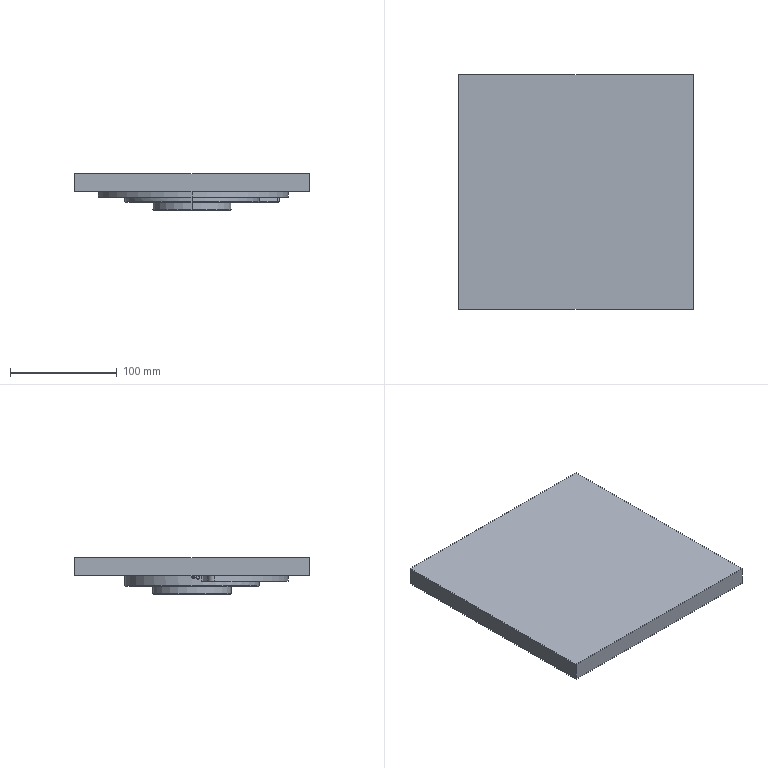NC program | NX | posted with a generic post | part box 220 x 220 x 34.5 mm
Lines 3232 to 4489 of 14163:
(ZLEVEL_PROFILE_COPY , TOOL : D10JING)
N6426 T07 M6
N6428 G54
N6430 G17 G0 G90 X93.952 Y24.124 S8000 M3
N6432 G43 Z30. H7
N6434 Z-17.
N6436 G94 G1 X92.706 Y22.948 F1200.
N6438 G3 X92.42 Y21.99 R1.
N6440 G1 X92.427 Y21.958
N6442 G2 X84.432 Y9.81 R10.
N6444 G1 X67.654 Y6.852
N6446 X67.704 Y6.339
N6448 G2 X-54.559 Y-40.587 R68.
N6450 G1 X-54.815 Y-40.238
N6452 X-54.822 Y-40.231
N6454 G2 X-56.208 Y-38.271 R68.
N6456 G1 X-56.229 Y-38.238
N6458 X-70.985 Y-46.757
N6460 G2 X-84.924 Y-42.578 R10.
N6462 G3 X-85.759 Y-42.028 R1.
N6464 G1 X-87.471 Y-41.927
N6466 G0 Z30.
N6468 M5
(ZLEVEL_PROFILE_COPY_1 , TOOL : D6)
N6470 T09 M6
N6472 G54
N6474 G17 G0 G90 X44.19 Y25.815 S9500 M3
N6476 G43 Z30. H9
N6478 Z-0.493
N6480 G94 G1 X43.248 Y26.254 F1000.
N6482 G3 X42.65 Y26.202 R0.6
N6484 G1 X40.963 Y25.02 F1500.
N6486 G2 X41.984 Y23.268 R48.
N6488 G3 X42.498 Y22.959 R0.6
N6490 G1 X43.512 Y22.941
N6492 G0 X44.19 Y25.815 Z-0.986
N6494 G1 X43.248 Y26.254 F1000.
N6496 G3 X42.65 Y26.202 R0.6
N6498 G1 X40.963 Y25.02 F1500.
N6500 G2 X41.984 Y23.268 R48.
N6502 G3 X42.498 Y22.959 R0.6
N6504 G1 X43.512 Y22.941
N6506 G0 X44.19 Y25.815 Z-1.479
N6508 G1 X43.248 Y26.254 F1000.
N6510 G3 X42.65 Y26.202 R0.6
N6512 G1 X40.963 Y25.02 F1500.
N6514 G2 X41.984 Y23.268 R48.
N6516 G3 X42.498 Y22.959 R0.6
N6518 G1 X43.512 Y22.941
N6520 G0 X44.19 Y25.815 Z-1.972
N6522 G1 X43.248 Y26.254 F1000.
N6524 G3 X42.65 Y26.202 R0.6
N6526 G1 X40.963 Y25.02 F1500.
N6528 G2 X41.984 Y23.268 R48.
N6530 G3 X42.498 Y22.959 R0.6
N6532 G1 X43.512 Y22.941
N6534 G0 X44.19 Y25.815 Z-2.465
N6536 G1 X43.248 Y26.254 F1000.
N6538 G3 X42.65 Y26.202 R0.6
N6540 G1 X40.963 Y25.02 F1500.
N6542 G2 X41.984 Y23.268 R48.
N6544 G3 X42.498 Y22.959 R0.6
N6546 G1 X43.512 Y22.941
N6548 G0 X44.19 Y25.815 Z-2.958
N6550 G1 X43.248 Y26.254 F1000.
N6552 G3 X42.65 Y26.202 R0.6
N6554 G1 X40.963 Y25.02 F1500.
N6556 G2 X41.984 Y23.268 R48.
N6558 G3 X42.498 Y22.959 R0.6
N6560 G1 X43.512 Y22.941
N6562 G0 X44.19 Y25.815 Z-3.451
N6564 G1 X43.248 Y26.254 F1000.
N6566 G3 X42.65 Y26.202 R0.6
N6568 G1 X40.963 Y25.02 F1500.
N6570 G2 X41.984 Y23.268 R48.
N6572 G3 X42.498 Y22.959 R0.6
N6574 G1 X43.512 Y22.941
N6576 G0 X44.19 Y25.815 Z-3.944
N6578 G1 X43.248 Y26.254 F1000.
N6580 G3 X42.65 Y26.202 R0.6
N6582 G1 X40.963 Y25.02 F1500.
N6584 G2 X41.984 Y23.268 R48.
N6586 G3 X42.498 Y22.959 R0.6
N6588 G1 X43.512 Y22.941
N6590 G0 X44.19 Y25.815 Z-4.438
N6592 G1 X43.248 Y26.254 F1000.
N6594 G3 X42.65 Y26.202 R0.6
N6596 G1 X40.963 Y25.02 F1500.
N6598 G2 X41.984 Y23.268 R48.
N6600 G3 X42.498 Y22.959 R0.6
N6602 G1 X43.512 Y22.941
N6604 G0 X44.19 Y25.815 Z-4.931
N6606 G1 X43.248 Y26.254 F1000.
N6608 G3 X42.65 Y26.202 R0.6
N6610 G1 X40.963 Y25.02 F1500.
N6612 G2 X41.984 Y23.268 R48.
N6614 G3 X42.498 Y22.959 R0.6
N6616 G1 X43.512 Y22.941
N6618 G0 X44.19 Y25.815 Z-5.424
N6620 G1 X43.248 Y26.254 F1000.
N6622 G3 X42.65 Y26.202 R0.6
N6624 G1 X40.963 Y25.02 F1500.
N6626 G2 X41.984 Y23.268 R48.
N6628 G3 X42.498 Y22.959 R0.6
N6630 G1 X43.512 Y22.941
N6632 G0 X44.19 Y25.815 Z-5.917
N6634 G1 X43.248 Y26.254 F1000.
N6636 G3 X42.65 Y26.202 R0.6
N6638 G1 X40.963 Y25.02 F1500.
N6640 G2 X41.984 Y23.268 R48.
N6642 G3 X42.498 Y22.959 R0.6
N6644 G1 X43.512 Y22.941
N6646 G0 X44.19 Y25.815 Z-6.41
N6648 G1 X43.248 Y26.254 F1000.
N6650 G3 X42.65 Y26.202 R0.6
N6652 G1 X40.963 Y25.02 F1500.
N6654 G2 X41.984 Y23.268 R48.
N6656 G3 X42.498 Y22.959 R0.6
N6658 G1 X43.512 Y22.941
N6660 G0 X44.19 Y25.815 Z-6.903
N6662 G1 X43.248 Y26.254 F1000.
N6664 G3 X42.65 Y26.202 R0.6
N6666 G1 X40.963 Y25.02 F1500.
N6668 G2 X41.984 Y23.268 R48.
N6670 G3 X42.498 Y22.959 R0.6
N6672 G1 X43.512 Y22.941
N6674 G0 X44.19 Y25.815 Z-7.396
N6676 G1 X43.248 Y26.254 F1000.
N6678 G3 X42.65 Y26.202 R0.6
N6680 G1 X40.963 Y25.02 F1500.
N6682 G2 X41.984 Y23.268 R48.
N6684 G3 X42.498 Y22.959 R0.6
N6686 G1 X43.512 Y22.941
N6688 G0 X44.19 Y25.815 Z-7.889
N6690 G1 X43.248 Y26.254 F1000.
N6692 G3 X42.65 Y26.202 R0.6
N6694 G1 X40.963 Y25.02 F1500.
N6696 G2 X41.984 Y23.268 R48.
N6698 G3 X42.498 Y22.959 R0.6
N6700 G1 X43.512 Y22.941
N6702 G0 X44.19 Y25.815 Z-8.382
N6704 G1 X43.248 Y26.254 F1000.
N6706 G3 X42.65 Y26.202 R0.6
N6708 G1 X40.963 Y25.02 F1500.
N6710 G2 X41.984 Y23.268 R48.
N6712 G3 X42.498 Y22.959 R0.6
N6714 G1 X43.512 Y22.941
N6716 G0 X44.19 Y25.815 Z-8.875
N6718 G1 X43.248 Y26.254 F1000.
N6720 G3 X42.65 Y26.202 R0.6
N6722 G1 X40.963 Y25.02 F1500.
N6724 G2 X41.984 Y23.268 R48.
N6726 G3 X42.498 Y22.959 R0.6
N6728 G1 X43.512 Y22.941
N6730 G0 X44.19 Y25.815 Z-9.25
N6732 G1 X43.248 Y26.254 F1000.
N6734 G3 X42.65 Y26.202 R0.6
N6736 G1 X40.963 Y25.02 F1500.
N6738 G2 X41.984 Y23.268 R48.
N6740 G3 X42.498 Y22.959 R0.6
N6742 G1 X43.512 Y22.941
N6744 G0 X44.19 Y25.815 Z-9.625
N6746 G1 X43.248 Y26.254 F1000.
N6748 G3 X42.65 Y26.202 R0.6
N6750 G1 X40.963 Y25.02 F1500.
N6752 G2 X41.984 Y23.268 R48.
N6754 G3 X42.498 Y22.959 R0.6
N6756 G1 X43.512 Y22.941
N6758 G0 X44.19 Y25.815 Z-10.
N6760 G1 X43.248 Y26.254 F1000.
N6762 G3 X42.65 Y26.202 R0.6
N6764 G1 X40.963 Y25.02 F1500.
N6766 G2 X41.984 Y23.268 R48.
N6768 G3 X42.498 Y22.959 R0.6
N6770 G1 X43.512 Y22.941
N6772 G0 Z30.
N6774 X39.192 Y14.12
N6776 Z-0.493
N6778 G1 X38.335 Y14.707 F1000.
N6780 G3 X37.737 Y14.753 R0.6
N6782 G1 X35.912 Y13.878 F1500.
N6784 G2 X36.579 Y12.008 R38.5
N6786 G3 X37.027 Y11.608 R0.6
N6788 G1 X38.029 Y11.398
N6790 G0 X39.192 Y14.12 Z-0.986
N6792 G1 X38.335 Y14.707 F1000.
N6794 G3 X37.737 Y14.753 R0.6
N6796 G1 X35.912 Y13.878 F1500.
N6798 G2 X36.579 Y12.008 R38.5
N6800 G3 X37.026 Y11.608 R0.6
N6802 G1 X38.028 Y11.399
N6804 G0 X39.192 Y14.12 Z-1.479
N6806 G1 X38.335 Y14.707 F1000.
N6808 G3 X37.737 Y14.753 R0.6
N6810 G1 X35.912 Y13.878 F1500.
N6812 G2 X36.579 Y12.008 R38.5
N6814 G3 X37.026 Y11.608 R0.6
N6816 G1 X38.028 Y11.398
N6818 G0 X39.192 Y14.12 Z-1.972
N6820 G1 X38.335 Y14.707 F1000.
N6822 G3 X37.737 Y14.753 R0.6
N6824 G1 X35.912 Y13.878 F1500.
N6826 G2 X36.579 Y12.008 R38.5
N6828 G3 X37.026 Y11.608 R0.6
N6830 G1 X38.028 Y11.398
N6832 G0 X39.193 Y14.12 Z-2.465
N6834 G1 X38.335 Y14.707 F1000.
N6836 G3 X37.737 Y14.753 R0.6
N6838 G1 X35.912 Y13.878 F1500.
N6840 G2 X36.579 Y12.008 R38.5
N6842 G3 X37.026 Y11.608 R0.6
N6844 G1 X38.029 Y11.398
N6846 G0 X39.193 Y14.12 Z-2.958
N6848 G1 X38.335 Y14.707 F1000.
N6850 G3 X37.737 Y14.753 R0.6
N6852 G1 X35.912 Y13.878 F1500.
N6854 G2 X36.579 Y12.008 R38.5
N6856 G3 X37.026 Y11.608 R0.6
N6858 G1 X38.029 Y11.398
N6860 G0 X39.193 Y14.12 Z-3.451
N6862 G1 X38.335 Y14.707 F1000.
N6864 G3 X37.737 Y14.753 R0.6
N6866 G1 X35.912 Y13.878 F1500.
N6868 G2 X36.579 Y12.008 R38.5
N6870 G3 X37.027 Y11.608 R0.6
N6872 G1 X38.029 Y11.398
N6874 G0 X39.193 Y14.12 Z-3.944
N6876 G1 X38.335 Y14.707 F1000.
N6878 G3 X37.737 Y14.753 R0.6
N6880 G1 X35.912 Y13.878 F1500.
N6882 G2 X36.579 Y12.008 R38.5
N6884 G3 X37.027 Y11.608 R0.6
N6886 G1 X38.029 Y11.398
N6888 G0 X39.193 Y14.12 Z-4.438
N6890 G1 X38.335 Y14.707 F1000.
N6892 G3 X37.737 Y14.753 R0.6
N6894 G1 X35.912 Y13.878 F1500.
N6896 G2 X36.579 Y12.008 R38.5
N6898 G3 X37.027 Y11.608 R0.6
N6900 G1 X38.029 Y11.398
N6902 G0 X39.193 Y14.12 Z-4.931
N6904 G1 X38.335 Y14.707 F1000.
N6906 G3 X37.737 Y14.753 R0.6
N6908 G1 X35.912 Y13.878 F1500.
N6910 G2 X36.579 Y12.008 R38.5
N6912 G3 X37.027 Y11.608 R0.6
N6914 G1 X38.029 Y11.398
N6916 G0 X39.193 Y14.12 Z-5.424
N6918 G1 X38.335 Y14.707 F1000.
N6920 G3 X37.737 Y14.753 R0.6
N6922 G1 X35.912 Y13.878 F1500.
N6924 G2 X36.579 Y12.008 R38.5
N6926 G3 X37.027 Y11.608 R0.6
N6928 G1 X38.029 Y11.398
N6930 G0 X39.193 Y14.12 Z-5.917
N6932 G1 X38.335 Y14.707 F1000.
N6934 G3 X37.737 Y14.753 R0.6
N6936 G1 X35.912 Y13.878 F1500.
N6938 G2 X36.579 Y12.008 R38.5
N6940 G3 X37.027 Y11.608 R0.6
N6942 G1 X38.029 Y11.398
N6944 G0 X39.193 Y14.12 Z-6.41
N6946 G1 X38.335 Y14.707 F1000.
N6948 G3 X37.737 Y14.753 R0.6
N6950 G1 X35.912 Y13.878 F1500.
N6952 G2 X36.58 Y12.008 R38.5
N6954 G3 X37.027 Y11.608 R0.6
N6956 G1 X38.029 Y11.398
N6958 G0 X39.193 Y14.12 Z-6.903
N6960 G1 X38.336 Y14.707 F1000.
N6962 G3 X37.737 Y14.753 R0.6
N6964 G1 X35.912 Y13.878 F1500.
N6966 G2 X36.58 Y12.008 R38.5
N6968 G3 X37.027 Y11.608 R0.6
N6970 G1 X38.029 Y11.398
N6972 G0 X39.193 Y14.12 Z-7.396
N6974 G1 X38.336 Y14.707 F1000.
N6976 G3 X37.737 Y14.753 R0.6
N6978 G1 X35.912 Y13.878 F1500.
N6980 G2 X36.58 Y12.008 R38.5
N6982 G3 X37.027 Y11.608 R0.6
N6984 G1 X38.029 Y11.398
N6986 G0 X39.193 Y14.12 Z-7.889
N6988 G1 X38.336 Y14.707 F1000.
N6990 G3 X37.737 Y14.753 R0.6
N6992 G1 X35.912 Y13.878 F1500.
N6994 G2 X36.58 Y12.008 R38.5
N6996 G3 X37.027 Y11.608 R0.6
N6998 G1 X38.029 Y11.398
N7000 G0 X39.193 Y14.12 Z-8.382
N7002 G1 X38.336 Y14.707 F1000.
N7004 G3 X37.737 Y14.753 R0.6
N7006 G1 X35.912 Y13.878 F1500.
N7008 G2 X36.58 Y12.008 R38.5
N7010 G3 X37.027 Y11.608 R0.6
N7012 G1 X38.029 Y11.398
N7014 G0 X39.193 Y14.12 Z-8.875
N7016 G1 X38.336 Y14.707 F1000.
N7018 G3 X37.737 Y14.753 R0.6
N7020 G1 X35.912 Y13.878 F1500.
N7022 G2 X36.58 Y12.008 R38.5
N7024 G3 X37.027 Y11.608 R0.6
N7026 G1 X38.029 Y11.398
N7028 G0 X39.193 Y14.12 Z-9.25
N7030 G1 X38.336 Y14.707 F1000.
N7032 G3 X37.738 Y14.753 R0.6
N7034 G1 X35.912 Y13.878 F1500.
N7036 G2 X36.58 Y12.008 R38.5
N7038 G3 X37.027 Y11.608 R0.6
N7040 G1 X38.029 Y11.398
N7042 G0 X39.193 Y14.12 Z-9.625
N7044 G1 X38.336 Y14.707 F1000.
N7046 G3 X37.738 Y14.753 R0.6
N7048 G1 X35.912 Y13.878 F1500.
N7050 G2 X36.58 Y12.008 R38.5
N7052 G3 X37.027 Y11.607 R0.6
N7054 G1 X38.029 Y11.398
N7056 G0 X39.193 Y14.12 Z-10.
N7058 G1 X38.336 Y14.707 F1000.
N7060 G3 X37.738 Y14.753 R0.6
N7062 G1 X35.912 Y13.878 F1500.
N7064 G2 X36.58 Y12.008 R38.5
N7066 G3 X37.027 Y11.607 R0.6
N7068 G1 X38.029 Y11.398
N7070 G0 Z30.
N7072 X-11.399 Y-38.028
N7074 Z-0.493
N7076 G1 X-11.608 Y-37.026 F1000.
N7078 G3 X-12.009 Y-36.579 R0.6
N7080 G2 X-13.878 Y-35.912 R38.5 F1500.
N7082 G1 X-14.753 Y-37.737
N7084 G3 X-14.707 Y-38.335 R0.6
N7086 G1 X-14.12 Y-39.192
N7088 G0 X-11.399 Y-38.028 Z-0.986
N7090 G1 X-11.608 Y-37.026 F1000.
N7092 G3 X-12.009 Y-36.579 R0.6
N7094 G2 X-13.878 Y-35.912 R38.5 F1500.
N7096 G1 X-14.753 Y-37.737
N7098 G3 X-14.707 Y-38.335 R0.6
N7100 G1 X-14.12 Y-39.192
N7102 G0 X-11.399 Y-38.028 Z-1.479
N7104 G1 X-11.608 Y-37.026 F1000.
N7106 G3 X-12.009 Y-36.579 R0.6
N7108 G2 X-13.878 Y-35.912 R38.5 F1500.
N7110 G1 X-14.753 Y-37.737
N7112 G3 X-14.707 Y-38.335 R0.6
N7114 G1 X-14.12 Y-39.192
N7116 G0 X-11.399 Y-38.028 Z-1.972
N7118 G1 X-11.608 Y-37.026 F1000.
N7120 G3 X-12.009 Y-36.579 R0.6
N7122 G2 X-13.878 Y-35.912 R38.5 F1500.
N7124 G1 X-14.753 Y-37.737
N7126 G3 X-14.707 Y-38.335 R0.6
N7128 G1 X-14.12 Y-39.192
N7130 G0 X-11.399 Y-38.028 Z-2.465
N7132 G1 X-11.608 Y-37.026 F1000.
N7134 G3 X-12.009 Y-36.579 R0.6
N7136 G2 X-13.878 Y-35.912 R38.5 F1500.
N7138 G1 X-14.753 Y-37.737
N7140 G3 X-14.707 Y-38.335 R0.6
N7142 G1 X-14.12 Y-39.192
N7144 G0 X-11.399 Y-38.028 Z-2.958
N7146 G1 X-11.608 Y-37.026 F1000.
N7148 G3 X-12.009 Y-36.579 R0.6
N7150 G2 X-13.878 Y-35.912 R38.5 F1500.
N7152 G1 X-14.753 Y-37.737
N7154 G3 X-14.707 Y-38.335 R0.6
N7156 G1 X-14.12 Y-39.192
N7158 G0 X-11.399 Y-38.028 Z-3.451
N7160 G1 X-11.608 Y-37.026 F1000.
N7162 G3 X-12.009 Y-36.579 R0.6
N7164 G2 X-13.878 Y-35.912 R38.5 F1500.
N7166 G1 X-14.753 Y-37.737
N7168 G3 X-14.707 Y-38.335 R0.6
N7170 G1 X-14.12 Y-39.192
N7172 G0 X-11.399 Y-38.028 Z-3.944
N7174 G1 X-11.608 Y-37.026 F1000.
N7176 G3 X-12.009 Y-36.579 R0.6
N7178 G2 X-13.878 Y-35.912 R38.5 F1500.
N7180 G1 X-14.753 Y-37.737
N7182 G3 X-14.707 Y-38.335 R0.6
N7184 G1 X-14.12 Y-39.192
N7186 G0 X-11.399 Y-38.028 Z-4.438
N7188 G1 X-11.608 Y-37.026 F1000.
N7190 G3 X-12.009 Y-36.579 R0.6
N7192 G2 X-13.878 Y-35.912 R38.5 F1500.
N7194 G1 X-14.753 Y-37.737
N7196 G3 X-14.707 Y-38.335 R0.6
N7198 G1 X-14.12 Y-39.192
N7200 G0 X-11.399 Y-38.028 Z-4.931
N7202 G1 X-11.608 Y-37.026 F1000.
N7204 G3 X-12.009 Y-36.579 R0.6
N7206 G2 X-13.878 Y-35.912 R38.5 F1500.
N7208 G1 X-14.753 Y-37.737
N7210 G3 X-14.707 Y-38.335 R0.6
N7212 G1 X-14.12 Y-39.192
N7214 G0 X-11.399 Y-38.028 Z-5.424
N7216 G1 X-11.608 Y-37.026 F1000.
N7218 G3 X-12.009 Y-36.579 R0.6
N7220 G2 X-13.878 Y-35.912 R38.5 F1500.
N7222 G1 X-14.753 Y-37.737
N7224 G3 X-14.707 Y-38.335 R0.6
N7226 G1 X-14.12 Y-39.192
N7228 G0 X-11.399 Y-38.028 Z-5.917
N7230 G1 X-11.608 Y-37.026 F1000.
N7232 G3 X-12.009 Y-36.579 R0.6
N7234 G2 X-13.878 Y-35.912 R38.5 F1500.
N7236 G1 X-14.753 Y-37.737
N7238 G3 X-14.707 Y-38.335 R0.6
N7240 G1 X-14.12 Y-39.192
N7242 G0 X-11.399 Y-38.028 Z-6.41
N7244 G1 X-11.608 Y-37.026 F1000.
N7246 G3 X-12.009 Y-36.579 R0.6
N7248 G2 X-13.878 Y-35.912 R38.5 F1500.
N7250 G1 X-14.753 Y-37.737
N7252 G3 X-14.707 Y-38.335 R0.6
N7254 G1 X-14.12 Y-39.192
N7256 G0 X-11.399 Y-38.028 Z-6.903
N7258 G1 X-11.608 Y-37.026 F1000.
N7260 G3 X-12.009 Y-36.579 R0.6
N7262 G2 X-13.878 Y-35.912 R38.5 F1500.
N7264 G1 X-14.753 Y-37.737
N7266 G3 X-14.707 Y-38.335 R0.6
N7268 G1 X-14.12 Y-39.192
N7270 G0 X-11.399 Y-38.028 Z-7.396
N7272 G1 X-11.608 Y-37.026 F1000.
N7274 G3 X-12.009 Y-36.579 R0.6
N7276 G2 X-13.878 Y-35.912 R38.5 F1500.
N7278 G1 X-14.753 Y-37.737
N7280 G3 X-14.707 Y-38.335 R0.6
N7282 G1 X-14.12 Y-39.192
N7284 G0 X-11.399 Y-38.028 Z-7.889
N7286 G1 X-11.608 Y-37.026 F1000.
N7288 G3 X-12.009 Y-36.579 R0.6
N7290 G2 X-13.878 Y-35.912 R38.5 F1500.
N7292 G1 X-14.753 Y-37.737
N7294 G3 X-14.707 Y-38.335 R0.6
N7296 G1 X-14.12 Y-39.192
N7298 G0 X-11.399 Y-38.028 Z-8.382
N7300 G1 X-11.608 Y-37.026 F1000.
N7302 G3 X-12.009 Y-36.579 R0.6
N7304 G2 X-13.878 Y-35.912 R38.5 F1500.
N7306 G1 X-14.753 Y-37.737
N7308 G3 X-14.707 Y-38.335 R0.6
N7310 G1 X-14.12 Y-39.192
N7312 G0 X-11.399 Y-38.028 Z-8.875
N7314 G1 X-11.608 Y-37.026 F1000.
N7316 G3 X-12.009 Y-36.579 R0.6
N7318 G2 X-13.878 Y-35.912 R38.5 F1500.
N7320 G1 X-14.753 Y-37.737
N7322 G3 X-14.707 Y-38.335 R0.6
N7324 G1 X-14.12 Y-39.192
N7326 G0 X-11.399 Y-38.028 Z-9.25
N7328 G1 X-11.608 Y-37.026 F1000.
N7330 G3 X-12.009 Y-36.579 R0.6
N7332 G2 X-13.878 Y-35.912 R38.5 F1500.
N7334 G1 X-14.753 Y-37.737
N7336 G3 X-14.707 Y-38.335 R0.6
N7338 G1 X-14.12 Y-39.192
N7340 G0 X-11.399 Y-38.028 Z-9.625
N7342 G1 X-11.608 Y-37.026 F1000.
N7344 G3 X-12.009 Y-36.579 R0.6
N7346 G2 X-13.878 Y-35.912 R38.5 F1500.
N7348 G1 X-14.753 Y-37.737
N7350 G3 X-14.707 Y-38.335 R0.6
N7352 G1 X-14.12 Y-39.192
N7354 G0 X-11.399 Y-38.028 Z-10.
N7356 G1 X-11.608 Y-37.026 F1000.
N7358 G3 X-12.009 Y-36.579 R0.6
N7360 G2 X-13.878 Y-35.912 R38.5 F1500.
N7362 G1 X-14.753 Y-37.737
N7364 G3 X-14.707 Y-38.335 R0.6
N7366 G1 X-14.12 Y-39.192
N7368 G0 Z30.
N7370 X-34.692 Y-23.062
N7372 Z-0.493
N7374 G1 X-33.719 Y-23.428 F1000.
N7376 G3 X-33.127 Y-23.33 R0.6
N7378 G1 X-31.563 Y-22.045 F1500.
N7380 G2 X-32.658 Y-20.389 R38.5
N7382 G3 X-33.188 Y-20.107 R0.6
N7384 G1 X-34.211 Y-20.142
N7386 G0 X-34.692 Y-23.062 Z-0.986
N7388 G1 X-33.719 Y-23.428 F1000.
N7390 G3 X-33.127 Y-23.33 R0.6
N7392 G1 X-31.563 Y-22.045 F1500.
N7394 G2 X-32.658 Y-20.389 R38.5
N7396 G3 X-33.188 Y-20.107 R0.6
N7398 G1 X-34.211 Y-20.142
N7400 G0 X-34.692 Y-23.062 Z-1.479
N7402 G1 X-33.719 Y-23.428 F1000.
N7404 G3 X-33.127 Y-23.33 R0.6
N7406 G1 X-31.563 Y-22.045 F1500.
N7408 G2 X-32.658 Y-20.389 R38.5
N7410 G3 X-33.188 Y-20.107 R0.6
N7412 G1 X-34.211 Y-20.142
N7414 G0 X-34.692 Y-23.062 Z-1.972
N7416 G1 X-33.719 Y-23.428 F1000.
N7418 G3 X-33.127 Y-23.33 R0.6
N7420 G1 X-31.563 Y-22.045 F1500.
N7422 G2 X-32.658 Y-20.389 R38.5
N7424 G3 X-33.188 Y-20.107 R0.6
N7426 G1 X-34.211 Y-20.142
N7428 G0 X-34.692 Y-23.062 Z-2.465
N7430 G1 X-33.719 Y-23.428 F1000.
N7432 G3 X-33.127 Y-23.33 R0.6
N7434 G1 X-31.563 Y-22.045 F1500.
N7436 G2 X-32.658 Y-20.389 R38.5
N7438 G3 X-33.188 Y-20.107 R0.6
N7440 G1 X-34.211 Y-20.142
N7442 G0 X-34.692 Y-23.062 Z-2.958
N7444 G1 X-33.719 Y-23.428 F1000.
N7446 G3 X-33.127 Y-23.33 R0.6
N7448 G1 X-31.563 Y-22.045 F1500.
N7450 G2 X-32.658 Y-20.389 R38.5
N7452 G3 X-33.188 Y-20.107 R0.6
N7454 G1 X-34.211 Y-20.142
N7456 G0 X-34.692 Y-23.062 Z-3.451
N7458 G1 X-33.719 Y-23.428 F1000.
N7460 G3 X-33.127 Y-23.33 R0.6
N7462 G1 X-31.563 Y-22.045 F1500.
N7464 G2 X-32.658 Y-20.389 R38.5
N7466 G3 X-33.188 Y-20.107 R0.6
N7468 G1 X-34.211 Y-20.142
N7470 G0 X-34.692 Y-23.062 Z-3.944
N7472 G1 X-33.719 Y-23.428 F1000.
N7474 G3 X-33.127 Y-23.33 R0.6
N7476 G1 X-31.563 Y-22.045 F1500.
N7478 G2 X-32.658 Y-20.389 R38.5
N7480 G3 X-33.188 Y-20.107 R0.6
N7482 G1 X-34.211 Y-20.142
N7484 G0 X-34.692 Y-23.062 Z-4.438
N7486 G1 X-33.719 Y-23.428 F1000.
N7488 G3 X-33.127 Y-23.33 R0.6
N7490 G1 X-31.563 Y-22.045 F1500.
N7492 G2 X-32.658 Y-20.389 R38.5
N7494 G3 X-33.188 Y-20.107 R0.6
N7496 G1 X-34.211 Y-20.142
N7498 G0 X-34.692 Y-23.062 Z-4.931
N7500 G1 X-33.719 Y-23.428 F1000.
N7502 G3 X-33.127 Y-23.33 R0.6
N7504 G1 X-31.563 Y-22.045 F1500.
N7506 G2 X-32.658 Y-20.389 R38.5
N7508 G3 X-33.188 Y-20.107 R0.6
N7510 G1 X-34.211 Y-20.142
N7512 G0 X-34.692 Y-23.062 Z-5.424
N7514 G1 X-33.719 Y-23.428 F1000.
N7516 G3 X-33.127 Y-23.33 R0.6
N7518 G1 X-31.563 Y-22.045 F1500.
N7520 G2 X-32.658 Y-20.389 R38.5
N7522 G3 X-33.188 Y-20.107 R0.6
N7524 G1 X-34.211 Y-20.142
N7526 G0 X-34.692 Y-23.062 Z-5.917
N7528 G1 X-33.719 Y-23.428 F1000.
N7530 G3 X-33.127 Y-23.33 R0.6
N7532 G1 X-31.563 Y-22.045 F1500.
N7534 G2 X-32.658 Y-20.389 R38.5
N7536 G3 X-33.188 Y-20.107 R0.6
N7538 G1 X-34.211 Y-20.142
N7540 G0 X-34.692 Y-23.062 Z-6.41
N7542 G1 X-33.719 Y-23.428 F1000.
N7544 G3 X-33.127 Y-23.33 R0.6
N7546 G1 X-31.563 Y-22.045 F1500.
N7548 G2 X-32.658 Y-20.389 R38.5
N7550 G3 X-33.188 Y-20.107 R0.6
N7552 G1 X-34.211 Y-20.142
N7554 G0 X-34.692 Y-23.062 Z-6.903
N7556 G1 X-33.719 Y-23.428 F1000.
N7558 G3 X-33.127 Y-23.33 R0.6
N7560 G1 X-31.563 Y-22.045 F1500.
N7562 G2 X-32.658 Y-20.389 R38.5
N7564 G3 X-33.188 Y-20.107 R0.6
N7566 G1 X-34.211 Y-20.142
N7568 G0 X-34.692 Y-23.062 Z-7.396
N7570 G1 X-33.719 Y-23.428 F1000.
N7572 G3 X-33.127 Y-23.33 R0.6
N7574 G1 X-31.563 Y-22.045 F1500.
N7576 G2 X-32.658 Y-20.389 R38.5
N7578 G3 X-33.188 Y-20.107 R0.6
N7580 G1 X-34.211 Y-20.142
N7582 G0 X-34.692 Y-23.062 Z-7.889
N7584 G1 X-33.719 Y-23.428 F1000.
N7586 G3 X-33.127 Y-23.33 R0.6
N7588 G1 X-31.563 Y-22.045 F1500.
N7590 G2 X-32.658 Y-20.389 R38.5
N7592 G3 X-33.188 Y-20.107 R0.6
N7594 G1 X-34.211 Y-20.142
N7596 G0 X-34.692 Y-23.062 Z-8.382
N7598 G1 X-33.719 Y-23.428 F1000.
N7600 G3 X-33.127 Y-23.33 R0.6
N7602 G1 X-31.563 Y-22.045 F1500.
N7604 G2 X-32.658 Y-20.389 R38.5
N7606 G3 X-33.188 Y-20.107 R0.6
N7608 G1 X-34.211 Y-20.142
N7610 G0 X-34.692 Y-23.062 Z-8.875
N7612 G1 X-33.719 Y-23.428 F1000.
N7614 G3 X-33.127 Y-23.33 R0.6
N7616 G1 X-31.563 Y-22.045 F1500.
N7618 G2 X-32.658 Y-20.389 R38.5
N7620 G3 X-33.188 Y-20.107 R0.6
N7622 G1 X-34.211 Y-20.142
N7624 G0 X-34.692 Y-23.062 Z-9.25
N7626 G1 X-33.719 Y-23.428 F1000.
N7628 G3 X-33.127 Y-23.33 R0.6
N7630 G1 X-31.563 Y-22.045 F1500.
N7632 G2 X-32.658 Y-20.389 R38.5
N7634 G3 X-33.188 Y-20.107 R0.6
N7636 G1 X-34.211 Y-20.142
N7638 G0 X-34.692 Y-23.062 Z-9.625
N7640 G1 X-33.719 Y-23.428 F1000.
N7642 G3 X-33.127 Y-23.33 R0.6
N7644 G1 X-31.563 Y-22.045 F1500.
N7646 G2 X-32.658 Y-20.389 R38.5
N7648 G3 X-33.188 Y-20.107 R0.6
N7650 G1 X-34.211 Y-20.142
N7652 G0 X-34.692 Y-23.062 Z-10.
N7654 G1 X-33.719 Y-23.428 F1000.
N7656 G3 X-33.127 Y-23.33 R0.6
N7658 G1 X-31.563 Y-22.045 F1500.
N7660 G2 X-32.658 Y-20.389 R38.5
N7662 G3 X-33.188 Y-20.107 R0.6
N7664 G1 X-34.211 Y-20.142
N7666 G0 Z30.
N7668 X68.752 Y7.858
N7670 Z-0.493
N7672 G1 X68.084 Y8.654 F1000.
N7674 G3 X67.52 Y8.859 R0.6
N7676 G1 X65.451 Y8.495 F1500.
N7678 G2 X65.686 Y6.431 R66.
N7680 G3 X66.035 Y5.943 R0.6
N7682 G1 X66.973 Y5.517
N7684 G0 X68.752 Y7.858 Z-0.986
N7686 G1 X68.084 Y8.654 F1000.
N7688 G3 X67.52 Y8.859 R0.6
N7690 G1 X65.451 Y8.495 F1500.
N7692 G2 X65.686 Y6.431 R66.
N7694 G3 X66.035 Y5.943 R0.6
N7696 G1 X66.973 Y5.517
N7698 G0 X68.752 Y7.858 Z-1.479
N7700 G1 X68.084 Y8.654 F1000.
N7702 G3 X67.52 Y8.859 R0.6
N7704 G1 X65.451 Y8.495 F1500.
N7706 G2 X65.686 Y6.431 R66.
N7708 G3 X66.035 Y5.943 R0.6
N7710 G1 X66.973 Y5.517
N7712 G0 X68.752 Y7.858 Z-1.972
N7714 G1 X68.084 Y8.654 F1000.
N7716 G3 X67.52 Y8.859 R0.6
N7718 G1 X65.451 Y8.495 F1500.
N7720 G2 X65.686 Y6.431 R66.
N7722 G3 X66.035 Y5.943 R0.6
N7724 G1 X66.973 Y5.517
N7726 G0 X68.752 Y7.858 Z-2.465
N7728 G1 X68.084 Y8.654 F1000.
N7730 G3 X67.52 Y8.859 R0.6
N7732 G1 X65.451 Y8.495 F1500.
N7734 G2 X65.686 Y6.431 R66.
N7736 G3 X66.035 Y5.943 R0.6
N7738 G1 X66.973 Y5.517
N7740 G0 X68.752 Y7.858 Z-2.958
N7742 G1 X68.084 Y8.654 F1000.
N7744 G3 X67.52 Y8.859 R0.6
N7746 G1 X65.451 Y8.495 F1500.
N7748 G2 X65.686 Y6.431 R66.
N7750 G3 X66.035 Y5.943 R0.6
N7752 G1 X66.973 Y5.517
N7754 G0 X68.752 Y7.858 Z-3.451
N7756 G1 X68.084 Y8.654 F1000.
N7758 G3 X67.52 Y8.859 R0.6
N7760 G1 X65.451 Y8.495 F1500.
N7762 G2 X65.686 Y6.431 R66.
N7764 G3 X66.035 Y5.943 R0.6
N7766 G1 X66.973 Y5.517
N7768 G0 X68.752 Y7.858 Z-3.944
N7770 G1 X68.084 Y8.654 F1000.
N7772 G3 X67.52 Y8.859 R0.6
N7774 G1 X65.451 Y8.495 F1500.
N7776 G2 X65.686 Y6.431 R66.
N7778 G3 X66.035 Y5.943 R0.6
N7780 G1 X66.973 Y5.517
N7782 G0 X68.752 Y7.858 Z-4.438
N7784 G1 X68.084 Y8.654 F1000.
N7786 G3 X67.52 Y8.859 R0.6
N7788 G1 X65.451 Y8.495 F1500.
N7790 G2 X65.686 Y6.431 R66.
N7792 G3 X66.035 Y5.943 R0.6
N7794 G1 X66.973 Y5.517
N7796 G0 X68.752 Y7.858 Z-4.931
N7798 G1 X68.084 Y8.654 F1000.
N7800 G3 X67.52 Y8.859 R0.6
N7802 G1 X65.451 Y8.495 F1500.
N7804 G2 X65.686 Y6.431 R66.
N7806 G3 X66.035 Y5.943 R0.6
N7808 G1 X66.973 Y5.517
N7810 G0 X68.752 Y7.858 Z-5.424
N7812 G1 X68.084 Y8.654 F1000.
N7814 G3 X67.52 Y8.859 R0.6
N7816 G1 X65.451 Y8.495 F1500.
N7818 G2 X65.686 Y6.431 R66.
N7820 G3 X66.035 Y5.943 R0.6
N7822 G1 X66.973 Y5.517
N7824 G0 X68.752 Y7.858 Z-5.917
N7826 G1 X68.084 Y8.654 F1000.
N7828 G3 X67.52 Y8.859 R0.6
N7830 G1 X65.451 Y8.495 F1500.
N7832 G2 X65.686 Y6.431 R66.
N7834 G3 X66.035 Y5.943 R0.6
N7836 G1 X66.973 Y5.517
N7838 G0 X68.752 Y7.858 Z-6.41
N7840 G1 X68.084 Y8.654 F1000.
N7842 G3 X67.52 Y8.859 R0.6
N7844 G1 X65.451 Y8.495 F1500.
N7846 G2 X65.686 Y6.431 R66.
N7848 G3 X66.035 Y5.943 R0.6
N7850 G1 X66.973 Y5.517
N7852 G0 X68.752 Y7.858 Z-6.903
N7854 G1 X68.084 Y8.654 F1000.
N7856 G3 X67.52 Y8.859 R0.6
N7858 G1 X65.451 Y8.495 F1500.
N7860 G2 X65.686 Y6.431 R66.
N7862 G3 X66.035 Y5.943 R0.6
N7864 G1 X66.973 Y5.517
N7866 G0 X68.752 Y7.858 Z-7.396
N7868 G1 X68.084 Y8.654 F1000.
N7870 G3 X67.52 Y8.859 R0.6
N7872 G1 X65.451 Y8.495 F1500.
N7874 G2 X65.686 Y6.431 R66.
N7876 G3 X66.035 Y5.943 R0.6
N7878 G1 X66.973 Y5.517
N7880 G0 X68.752 Y7.858 Z-7.889
N7882 G1 X68.084 Y8.654 F1000.
N7884 G3 X67.52 Y8.859 R0.6
N7886 G1 X65.451 Y8.495 F1500.
N7888 G2 X65.686 Y6.431 R66.
N7890 G3 X66.035 Y5.943 R0.6
N7892 G1 X66.973 Y5.517
N7894 G0 X68.752 Y7.858 Z-8.382
N7896 G1 X68.084 Y8.654 F1000.
N7898 G3 X67.52 Y8.859 R0.6
N7900 G1 X65.451 Y8.495 F1500.
N7902 G2 X65.686 Y6.431 R66.
N7904 G3 X66.035 Y5.943 R0.6
N7906 G1 X66.973 Y5.517
N7908 G0 X68.752 Y7.858 Z-8.875
N7910 G1 X68.084 Y8.654 F1000.
N7912 G3 X67.52 Y8.859 R0.6
N7914 G1 X65.451 Y8.495 F1500.
N7916 G2 X65.686 Y6.431 R66.
N7918 G3 X66.035 Y5.943 R0.6
N7920 G1 X66.973 Y5.517
N7922 G0 X68.752 Y7.858 Z-9.25
N7924 G1 X68.084 Y8.654 F1000.
N7926 G3 X67.52 Y8.859 R0.6
N7928 G1 X65.451 Y8.495 F1500.
N7930 G2 X65.686 Y6.431 R66.
N7932 G3 X66.035 Y5.943 R0.6
N7934 G1 X66.973 Y5.517
N7936 G0 X68.752 Y7.858 Z-9.625
N7938 G1 X68.084 Y8.654 F1000.
N7940 G3 X67.52 Y8.859 R0.6
N7942 G1 X65.451 Y8.495 F1500.
N7944 G2 X65.686 Y6.431 R66.
N7946 G3 X66.035 Y5.943 R0.6
N7948 G1 X66.973 Y5.517
N7950 G0 X68.752 Y7.858 Z-10.
N7952 G1 X68.084 Y8.654 F1000.
N7954 G3 X67.52 Y8.859 R0.6
N7956 G1 X65.451 Y8.495 F1500.
N7958 G2 X65.686 Y6.431 R66.
N7960 G3 X66.035 Y5.943 R0.6
N7962 G1 X66.973 Y5.517
N7964 G0 X68.752 Y7.858 Z-10.5
N7966 G1 X68.084 Y8.654 F1000.
N7968 G3 X67.52 Y8.859 R0.6
N7970 G1 X65.451 Y8.495 F1500.
N7972 G2 X65.686 Y6.431 R66.
N7974 G3 X66.035 Y5.943 R0.6
N7976 G1 X66.973 Y5.517
N7978 G0 X68.752 Y7.858 Z-11.
N7980 G1 X68.084 Y8.654 F1000.
N7982 G3 X67.52 Y8.859 R0.6
N7984 G1 X65.451 Y8.495 F1500.
N7986 G2 X65.686 Y6.431 R66.
N7988 G3 X66.035 Y5.943 R0.6
N7990 G1 X66.973 Y5.517
N7992 G0 X68.752 Y7.858 Z-11.5
N7994 G1 X68.084 Y8.654 F1000.
N7996 G3 X67.52 Y8.859 R0.6
N7998 G1 X65.451 Y8.495 F1500.
N8000 G2 X65.686 Y6.431 R66.
N8002 G3 X66.035 Y5.943 R0.6
N8004 G1 X66.973 Y5.517
N8006 G0 X68.752 Y7.858 Z-12.
N8008 G1 X68.084 Y8.654 F1000.
N8010 G3 X67.52 Y8.859 R0.6
N8012 G1 X65.451 Y8.495 F1500.
N8014 G2 X65.686 Y6.431 R66.
N8016 G3 X66.035 Y5.943 R0.6
N8018 G1 X66.973 Y5.517
N8020 G0 X66.796 Y7.359 Z-12.5
N8022 G1 X66.015 Y8.289 F1000.
N8024 G3 X65.451 Y8.495 R0.6
N8026 G2 X65.686 Y6.431 R66. F1500.
N8028 G3 X66.035 Y5.943 R0.6
N8030 G1 X66.973 Y5.517
N8032 G0 X66.796 Y7.359 Z-13.
N8034 G1 X66.015 Y8.289 F1000.
N8036 G3 X65.451 Y8.495 R0.6
N8038 G2 X65.686 Y6.431 R66. F1500.
N8040 G3 X66.035 Y5.943 R0.6
N8042 G1 X66.973 Y5.517
N8044 G0 X66.796 Y7.359 Z-13.5
N8046 G1 X66.015 Y8.289 F1000.
N8048 G3 X65.451 Y8.495 R0.6
N8050 G2 X65.686 Y6.431 R66. F1500.
N8052 G3 X66.035 Y5.943 R0.6
N8054 G1 X66.973 Y5.517
N8056 G0 X66.796 Y7.359 Z-14.
N8058 G1 X66.015 Y8.289 F1000.
N8060 G3 X65.451 Y8.495 R0.6
N8062 G2 X65.686 Y6.431 R66. F1500.
N8064 G3 X66.035 Y5.943 R0.6
N8066 G1 X66.973 Y5.517
N8068 G0 X66.796 Y7.359 Z-14.5
N8070 G1 X66.015 Y8.289 F1000.
N8072 G3 X65.451 Y8.495 R0.6
N8074 G2 X65.686 Y6.431 R66. F1500.
N8076 G3 X66.035 Y5.943 R0.6
N8078 G1 X66.973 Y5.517
N8080 G0 X66.796 Y7.359 Z-15.
N8082 G1 X66.015 Y8.289 F1000.
N8084 G3 X65.451 Y8.495 R0.6
N8086 G2 X65.686 Y6.431 R66. F1500.
N8088 G3 X66.035 Y5.943 R0.6
N8090 G1 X66.973 Y5.517
N8092 G0 X66.796 Y7.359 Z-15.5
N8094 G1 X66.015 Y8.289 F1000.
N8096 G3 X65.451 Y8.495 R0.6
N8098 G2 X65.686 Y6.431 R66. F1500.
N8100 G3 X66.035 Y5.943 R0.6
N8102 G1 X66.973 Y5.517
N8104 G0 X66.796 Y7.359 Z-16.
N8106 G1 X66.015 Y8.289 F1000.
N8108 G3 X65.451 Y8.495 R0.6
N8110 G2 X65.686 Y6.431 R66. F1500.
N8112 G3 X66.035 Y5.943 R0.6
N8114 G1 X66.973 Y5.517
N8116 G0 X66.796 Y7.359 Z-16.5
N8118 G1 X66.015 Y8.289 F1000.
N8120 G3 X65.451 Y8.495 R0.6
N8122 G2 X65.686 Y6.431 R66. F1500.
N8124 G3 X66.035 Y5.943 R0.6
N8126 G1 X66.973 Y5.517
N8128 G0 Z30.
N8130 X-54.851 Y-38.823
N8132 Z-0.493
N8134 G1 X-54.406 Y-37.894 F1000.
N8136 G3 X-54.452 Y-37.296 R0.6
N8138 G2 X-55.599 Y-35.564 R66. F1500.
N8140 G1 X-57.418 Y-36.614
N8142 G3 X-57.718 Y-37.134 R0.6
N8144 G1 Y-38.173
N8146 G0 X-54.851 Y-38.823 Z-0.986
N8148 G1 X-54.406 Y-37.894 F1000.
N8150 G3 X-54.452 Y-37.296 R0.6
N8152 G2 X-55.599 Y-35.564 R66. F1500.
N8154 G1 X-57.418 Y-36.614
N8156 G3 X-57.718 Y-37.134 R0.6
N8158 G1 Y-38.173
N8160 G0 X-54.851 Y-38.823 Z-1.479
N8162 G1 X-54.406 Y-37.894 F1000.
N8164 G3 X-54.452 Y-37.296 R0.6
N8166 G2 X-55.599 Y-35.564 R66. F1500.
N8168 G1 X-57.418 Y-36.614
N8170 G3 X-57.718 Y-37.134 R0.6
N8172 G1 Y-38.173
N8174 G0 X-54.851 Y-38.823 Z-1.972
N8176 G1 X-54.406 Y-37.894 F1000.
N8178 G3 X-54.452 Y-37.296 R0.6
N8180 G2 X-55.599 Y-35.564 R66. F1500.
N8182 G1 X-57.418 Y-36.614
N8184 G3 X-57.718 Y-37.134 R0.6
N8186 G1 Y-38.173
N8188 G0 X-54.851 Y-38.823 Z-2.465
N8190 G1 X-54.406 Y-37.894 F1000.
N8192 G3 X-54.452 Y-37.296 R0.6
N8194 G2 X-55.599 Y-35.564 R66. F1500.
N8196 G1 X-57.418 Y-36.614
N8198 G3 X-57.718 Y-37.134 R0.6
N8200 G1 Y-38.173
N8202 G0 X-54.851 Y-38.823 Z-2.958
N8204 G1 X-54.406 Y-37.894 F1000.
N8206 G3 X-54.452 Y-37.296 R0.6
N8208 G2 X-55.599 Y-35.564 R66. F1500.
N8210 G1 X-57.418 Y-36.614
N8212 G3 X-57.718 Y-37.134 R0.6
N8214 G1 Y-38.173
N8216 G0 X-54.851 Y-38.823 Z-3.451
N8218 G1 X-54.406 Y-37.894 F1000.
N8220 G3 X-54.452 Y-37.296 R0.6
N8222 G2 X-55.599 Y-35.564 R66. F1500.
N8224 G1 X-57.418 Y-36.614
N8226 G3 X-57.718 Y-37.134 R0.6
N8228 G1 Y-38.173
N8230 G0 X-54.851 Y-38.823 Z-3.944
N8232 G1 X-54.406 Y-37.894 F1000.
N8234 G3 X-54.452 Y-37.296 R0.6
N8236 G2 X-55.599 Y-35.564 R66. F1500.
N8238 G1 X-57.418 Y-36.614
N8240 G3 X-57.718 Y-37.134 R0.6
N8242 G1 Y-38.173
N8244 G0 X-54.851 Y-38.823 Z-4.438
N8246 G1 X-54.406 Y-37.894 F1000.
N8248 G3 X-54.452 Y-37.296 R0.6
N8250 G2 X-55.599 Y-35.564 R66. F1500.
N8252 G1 X-57.418 Y-36.614
N8254 G3 X-57.718 Y-37.134 R0.6
N8256 G1 Y-38.173
N8258 G0 X-54.851 Y-38.823 Z-4.931
N8260 G1 X-54.406 Y-37.894 F1000.
N8262 G3 X-54.452 Y-37.296 R0.6
N8264 G2 X-55.599 Y-35.564 R66. F1500.
N8266 G1 X-57.418 Y-36.614
N8268 G3 X-57.718 Y-37.134 R0.6
N8270 G1 Y-38.173
N8272 G0 X-54.851 Y-38.823 Z-5.424
N8274 G1 X-54.406 Y-37.894 F1000.
N8276 G3 X-54.452 Y-37.296 R0.6
N8278 G2 X-55.599 Y-35.564 R66. F1500.
N8280 G1 X-57.418 Y-36.614
N8282 G3 X-57.718 Y-37.134 R0.6
N8284 G1 Y-38.173
N8286 G0 X-54.851 Y-38.823 Z-5.917
N8288 G1 X-54.406 Y-37.894 F1000.
N8290 G3 X-54.452 Y-37.296 R0.6
N8292 G2 X-55.599 Y-35.564 R66. F1500.
N8294 G1 X-57.418 Y-36.614
N8296 G3 X-57.718 Y-37.134 R0.6
N8298 G1 Y-38.173
N8300 G0 X-54.851 Y-38.823 Z-6.41
N8302 G1 X-54.406 Y-37.894 F1000.
N8304 G3 X-54.452 Y-37.296 R0.6
N8306 G2 X-55.599 Y-35.564 R66. F1500.
N8308 G1 X-57.418 Y-36.614
N8310 G3 X-57.718 Y-37.134 R0.6
N8312 G1 Y-38.173
N8314 G0 X-54.851 Y-38.823 Z-6.903
N8316 G1 X-54.406 Y-37.894 F1000.
N8318 G3 X-54.452 Y-37.296 R0.6
N8320 G2 X-55.599 Y-35.564 R66. F1500.
N8322 G1 X-57.418 Y-36.614
N8324 G3 X-57.718 Y-37.134 R0.6
N8326 G1 Y-38.173
N8328 G0 X-54.851 Y-38.823 Z-7.396
N8330 G1 X-54.406 Y-37.894 F1000.
N8332 G3 X-54.452 Y-37.296 R0.6
N8334 G2 X-55.599 Y-35.564 R66. F1500.
N8336 G1 X-57.418 Y-36.614
N8338 G3 X-57.718 Y-37.134 R0.6
N8340 G1 Y-38.173
N8342 G0 X-54.851 Y-38.823 Z-7.889
N8344 G1 X-54.406 Y-37.894 F1000.
N8346 G3 X-54.452 Y-37.296 R0.6
N8348 G2 X-55.599 Y-35.564 R66. F1500.
N8350 G1 X-57.418 Y-36.614
N8352 G3 X-57.718 Y-37.134 R0.6
N8354 G1 Y-38.173
N8356 G0 X-54.851 Y-38.823 Z-8.382
N8358 G1 X-54.406 Y-37.894 F1000.
N8360 G3 X-54.452 Y-37.296 R0.6
N8362 G2 X-55.599 Y-35.564 R66. F1500.
N8364 G1 X-57.418 Y-36.614
N8366 G3 X-57.718 Y-37.134 R0.6
N8368 G1 Y-38.173
N8370 G0 X-54.851 Y-38.823 Z-8.875
N8372 G1 X-54.406 Y-37.894 F1000.
N8374 G3 X-54.452 Y-37.296 R0.6
N8376 G2 X-55.599 Y-35.564 R66. F1500.
N8378 G1 X-57.418 Y-36.614
N8380 G3 X-57.718 Y-37.134 R0.6
N8382 G1 Y-38.173
N8384 G0 X-54.851 Y-38.823 Z-9.25
N8386 G1 X-54.406 Y-37.894 F1000.
N8388 G3 X-54.452 Y-37.296 R0.6
N8390 G2 X-55.599 Y-35.564 R66. F1500.
N8392 G1 X-57.418 Y-36.614
N8394 G3 X-57.718 Y-37.134 R0.6
N8396 G1 Y-38.173
N8398 G0 X-54.851 Y-38.823 Z-9.625
N8400 G1 X-54.406 Y-37.894 F1000.
N8402 G3 X-54.452 Y-37.296 R0.6
N8404 G2 X-55.599 Y-35.564 R66. F1500.
N8406 G1 X-57.418 Y-36.614
N8408 G3 X-57.718 Y-37.134 R0.6
N8410 G1 Y-38.173
N8412 G0 X-54.851 Y-38.823 Z-10.
N8414 G1 X-54.406 Y-37.894 F1000.
N8416 G3 X-54.452 Y-37.296 R0.6
N8418 G2 X-55.599 Y-35.564 R66. F1500.
N8420 G1 X-57.418 Y-36.614
N8422 G3 X-57.718 Y-37.134 R0.6
N8424 G1 Y-38.173
N8426 G0 X-54.851 Y-38.823 Z-10.5
N8428 G1 X-54.406 Y-37.894 F1000.
N8430 G3 X-54.452 Y-37.296 R0.6
N8432 G2 X-55.599 Y-35.564 R66. F1500.
N8434 G1 X-57.418 Y-36.614
N8436 G3 X-57.718 Y-37.134 R0.6
N8438 G1 Y-38.173
N8440 G0 X-54.851 Y-38.823 Z-11.
N8442 G1 X-54.406 Y-37.894 F1000.
N8444 G3 X-54.452 Y-37.296 R0.6
N8446 G2 X-55.599 Y-35.564 R66. F1500.
N8448 G1 X-57.418 Y-36.614
N8450 G3 X-57.718 Y-37.134 R0.6
N8452 G1 Y-38.173
N8454 G0 X-54.851 Y-38.823 Z-11.5
N8456 G1 X-54.406 Y-37.894 F1000.
N8458 G3 X-54.452 Y-37.296 R0.6
N8460 G2 X-55.599 Y-35.564 R66. F1500.
N8462 G1 X-57.418 Y-36.614
N8464 G3 X-57.718 Y-37.134 R0.6
N8466 G1 Y-38.173
N8468 G0 X-54.851 Y-38.823 Z-12.
N8470 G1 X-54.406 Y-37.894 F1000.
N8472 G3 X-54.452 Y-37.296 R0.6
N8474 G2 X-55.599 Y-35.564 R66. F1500.
N8476 G1 X-57.418 Y-36.614
N8478 G3 X-57.718 Y-37.134 R0.6
N8480 G1 Y-38.173
N8482 G0 X-54.851 Y-38.823 Z-12.5
N8484 G1 X-54.406 Y-37.894 F1000.
N8486 G3 X-54.452 Y-37.296 R0.6
N8488 G2 X-55.599 Y-35.564 R66. F1500.
N8490 G1 X-57.418 Y-36.614
N8492 G3 X-57.718 Y-37.134 R0.6
N8494 G1 Y-38.173
N8496 G0 X-54.851 Y-38.823 Z-13.
N8498 G1 X-54.406 Y-37.894 F1000.
N8500 G3 X-54.452 Y-37.296 R0.6
N8502 G2 X-55.599 Y-35.564 R66. F1500.
N8504 G1 X-57.418 Y-36.614
N8506 G3 X-57.718 Y-37.134 R0.6
N8508 G1 Y-38.173
N8510 G0 X-54.851 Y-38.823 Z-13.5
N8512 G1 X-54.406 Y-37.894 F1000.
N8514 G3 X-54.452 Y-37.296 R0.6
N8516 G2 X-55.599 Y-35.564 R66. F1500.
N8518 G1 X-57.418 Y-36.614
N8520 G3 X-57.718 Y-37.134 R0.6
N8522 G1 Y-38.173
N8524 G0 X-54.851 Y-38.823 Z-14.
N8526 G1 X-54.406 Y-37.894 F1000.
N8528 G3 X-54.452 Y-37.296 R0.6
N8530 G2 X-55.599 Y-35.564 R66. F1500.
N8532 G1 X-57.418 Y-36.614
N8534 G3 X-57.718 Y-37.134 R0.6
N8536 G1 Y-38.173
N8538 G0 X-54.851 Y-38.823 Z-14.5
N8540 G1 X-54.406 Y-37.894 F1000.
N8542 G3 X-54.452 Y-37.296 R0.6
N8544 G2 X-55.599 Y-35.564 R66. F1500.
N8546 G1 X-57.418 Y-36.614
N8548 G3 X-57.718 Y-37.134 R0.6
N8550 G1 Y-38.173
N8552 G0 X-54.851 Y-38.823 Z-15.
N8554 G1 X-54.406 Y-37.894 F1000.
N8556 G3 X-54.452 Y-37.296 R0.6
N8558 G2 X-55.599 Y-35.564 R66. F1500.
N8560 G1 X-57.418 Y-36.614
N8562 G3 X-57.718 Y-37.134 R0.6
N8564 G1 Y-38.173
N8566 G0 X-54.851 Y-38.823 Z-15.5
N8568 G1 X-54.406 Y-37.894 F1000.
N8570 G3 X-54.452 Y-37.296 R0.6
N8572 G2 X-55.599 Y-35.564 R66. F1500.
N8574 G1 X-57.418 Y-36.614
N8576 G3 X-57.718 Y-37.134 R0.6
N8578 G1 Y-38.173
N8580 G0 X-54.851 Y-38.823 Z-16.
N8582 G1 X-54.406 Y-37.894 F1000.
N8584 G3 X-54.452 Y-37.296 R0.6
N8586 G2 X-55.599 Y-35.564 R66. F1500.
N8588 G1 X-57.418 Y-36.614
N8590 G3 X-57.718 Y-37.134 R0.6
N8592 G1 Y-38.173
N8594 G0 X-54.851 Y-38.823 Z-16.5
N8596 G1 X-54.406 Y-37.894 F1000.
N8598 G3 X-54.452 Y-37.296 R0.6
N8600 G2 X-55.599 Y-35.564 R66. F1500.
N8602 G1 X-57.418 Y-36.614
N8604 G3 X-57.718 Y-37.134 R0.6
N8606 G1 Y-38.173
N8608 G0 Z30.
(FLOOR_WALL , TOOL : D6)
N8610 X49.256 Y-0.886
N8612 Z-8.5
N8614 G1 Z-10. F1000.
N8616 G3 X50. Y0. R0.9
N8618 X49.869 Y3.616 R50.
N8620 X49.739 Y5.099 R50.
N8622 X48.195 Y13.312 R50.
N8624 G2 X44.895 Y10.021 R12.5
N8626 X-10.021 Y-44.895 R46.
N8628 X-13.312 Y-48.195 R12.5
N8630 G3 X50. Y0. R50.
N8632 G1 X53.6
N8634 G3 X53.321 Y5.466 R53.6
N8636 X47.499 Y24.836 R53.6
N8638 G1 X46.068 Y23.834
N8640 G2 X42.088 Y12.524 R8.9
N8642 X41.718 Y12.336 R8.9
N8644 G1 X40.71 Y11.853
N8646 G2 X-11.853 Y-40.71 R42.4
N8648 G1 X-12.336 Y-41.718
N8650 G2 X-24.208 Y-45.9 R8.9
N8652 X-24.577 Y-45.712 R8.9
N8654 X-38.528 Y-34.773 R51.9
N8656 X-37.884 Y-22.203 R8.9
N8658 X-37.571 Y-21.933 R8.9
N8660 G1 X-36.706 Y-21.223
N8662 G2 X-36.952 Y-20.792 R42.4
N8664 G1 X-47.589 Y-24.664
N8666 G3 X-42.607 Y-32.521 R53.6
N8668 X-41.164 Y-34.329 R53.6
N8670 X53.6 Y0. R53.6
N8672 G1 X57.2
N8674 G3 X56.902 Y5.833 R57.2
N8676 X49.621 Y28.454 R57.2
N8678 X47.171 Y29.001 R1.7
N8680 G1 X41.365 Y24.936
N8682 G2 X42.541 Y22.872 R48.3
N8684 X40.383 Y15.694 R5.3
N8686 X40.163 Y15.583 R5.3
N8688 G1 X36.29 Y13.727
N8690 G2 X-13.727 Y-36.29 R38.8
N8692 G1 X-15.583 Y-40.163
N8694 G2 X-22.652 Y-42.653 R5.3
N8696 X-22.872 Y-42.541 R5.3
N8698 X-35.856 Y-32.361 R48.3
N8700 X-35.472 Y-24.876 R5.3
N8702 X-35.286 Y-24.715 R5.3
N8704 G1 X-31.968 Y-21.989
N8706 G2 X-34.543 Y-17.67 R38.8
N8708 G3 X-36.638 Y-16.847 R1.7
N8710 G1 X-50.812 Y-22.006
N8712 G3 X-51.769 Y-24.326 R1.7
N8714 X57.2 Y0. R57.2
N8716 G1 X56.756 Y-0.886
N8718 G3 X57.5 Y0. R0.9
N8720 X57.2 Y5.864 R57.5
N8722 X49.881 Y28.603 R57.5
N8724 X46.999 Y29.247 R2.
N8726 G1 X40.963 Y25.02
N8728 G2 X42.277 Y22.73 R48.
N8730 X40.241 Y15.959 R5.
N8732 X40.033 Y15.853 R5.
N8734 G1 X35.912 Y13.878
N8736 G2 X-13.878 Y-35.912 R38.5
N8738 G1 X-15.853 Y-40.033
N8740 G2 X-22.523 Y-42.382 R5.
N8742 X-22.73 Y-42.277 R5.
N8744 X-35.633 Y-32.16 R48.
N8746 X-35.095 Y-24.946 R5.
N8748 G1 X-31.563 Y-22.045
N8750 G2 X-34.276 Y-17.533 R38.5
N8752 G3 X-36.74 Y-16.565 R2.
N8754 G1 X-50.915 Y-21.724
N8756 G3 X-52.041 Y-24.454 R2.
N8758 X57.5 Y0. R57.5
N8760 X56.756 Y0.886 R0.9
N8762 G1 X55.991 Y1.021
N8764 Z-8.5
N8766 G0 Z30.
(HOLE_MILLING , TOOL : D6)
N8768 X36. Y38.5
N8770 Z0.5
N8772 G3 X35.3 Y39.2 R0.7 F1300.
N8774 X34.6 Y38.5 R0.7
N8776 X34.6 Y38.5 Z0.1 I1.4 J0.
N8778 X34.6 Y38.5 Z-0.3 I1.4 J0.
N8780 X34.6 Y38.5 Z-0.7 I1.4 J0.
N8782 X34.6 Y38.5 Z-1.1 I1.4 J0.
N8784 X34.6 Y38.5 Z-1.5 I1.4 J0.
N8786 X34.6 Y38.5 Z-1.9 I1.4 J0.
N8788 X34.6 Y38.5 Z-2.3 I1.4 J0.
N8790 X34.6 Y38.5 Z-2.7 I1.4 J0.
N8792 X34.6 Y38.5 Z-3.1 I1.4 J0.
N8794 X34.6 Y38.5 Z-3.5 I1.4 J0.
N8796 X34.6 Y38.5 Z-3.9 I1.4 J0.
N8798 X34.6 Y38.5 Z-4.3 I1.4 J0.
N8800 X34.6 Y38.5 Z-4.7 I1.4 J0.
N8802 X34.6 Y38.5 Z-5.1 I1.4 J0.
N8804 X34.6 Y38.5 Z-5.5 I1.4 J0.
N8806 X34.6 Y38.5 Z-5.9 I1.4 J0.
N8808 X34.6 Y38.5 Z-6.3 I1.4 J0.
N8810 X34.6 Y38.5 Z-6.7 I1.4 J0.
N8812 X34.6 Y38.5 Z-7.1 I1.4 J0.
N8814 X34.6 Y38.5 Z-7.5 I1.4 J0.
N8816 X34.6 Y38.5 Z-7.9 I1.4 J0.
N8818 X34.6 Y38.5 Z-8.3 I1.4 J0.
N8820 X34.6 Y38.5 Z-8.7 I1.4 J0.
N8822 X34.6 Y38.5 Z-9.1 I1.4 J0.
N8824 X34.6 Y38.5 Z-9.5 I1.4 J0.
N8826 X34.6 Y38.5 Z-9.9 I1.4 J0.
N8828 X34.6 Y38.5 Z-10.3 I1.4 J0.
N8830 X34.6 Y38.5 Z-10.7 I1.4 J0.
N8832 X34.6 Y38.5 Z-11.1 I1.4 J0.
N8834 X34.6 Y38.5 Z-11.5 I1.4 J0.
N8836 X34.6 Y38.5 Z-11.9 I1.4 J0.
N8838 X34.6 Y38.5 Z-12.3 I1.4 J0.
N8840 X34.6 Y38.5 Z-12.7 I1.4 J0.
N8842 X34.6 Y38.5 Z-13.1 I1.4 J0.
N8844 X34.6 Y38.5 Z-13.5 I1.4 J0.
N8846 X34.6 Y38.5 Z-13.9 I1.4 J0.
N8848 X34.6 Y38.5 Z-14.3 I1.4 J0.
N8850 X34.6 Y38.5 Z-14.7 I1.4 J0.
N8852 X34.6 Y38.5 Z-15.1 I1.4 J0.
N8854 X34.6 Y38.5 Z-15.5 I1.4 J0.
N8856 X34.6 Y38.5 Z-15.9 I1.4 J0.
N8858 X34.6 Y38.5 Z-16.3 I1.4 J0.
N8860 X34.6 Y38.5 Z-16.7 I1.4 J0.
N8862 X36. Y39.9 Z-17. R-1.4
N8864 X34.6 Y38.5 R1.4
N8866 X36. Y39.9 R-1.4
N8868 X35.3 Y39.2 R0.7
N8870 X36. Y38.5 R0.7
N8872 G0 Z30.
N8874 X-36.641 Y-37.599
N8876 Z-9.5
N8878 G3 X-37.091 Y-37.149 R0.45
N8880 X-37.541 Y-37.599 R0.45
N8882 X-37.541 Y-37.599 Z-9.9 I0.9 J0.
N8884 X-37.541 Y-37.599 Z-10.3 I0.9 J0.
N8886 X-37.541 Y-37.599 Z-10.7 I0.9 J0.
N8888 X-37.541 Y-37.599 Z-11.1 I0.9 J0.
N8890 X-37.541 Y-37.599 Z-11.5 I0.9 J0.
N8892 X-37.541 Y-37.599 Z-11.9 I0.9 J0.
N8894 X-37.541 Y-37.599 Z-12.3 I0.9 J0.
N8896 X-37.541 Y-37.599 Z-12.7 I0.9 J0.
N8898 X-37.541 Y-37.599 Z-13.1 I0.9 J0.
N8900 X-37.541 Y-37.599 Z-13.5 I0.9 J0.
N8902 X-37.541 Y-37.599 Z-13.9 I0.9 J0.
N8904 X-36.641 Y-38.499 Z-14. R0.9
N8906 X-35.741 Y-37.599 R0.9
N8908 X-36.641 Y-38.499 R-0.9
N8910 X-36.191 Y-38.049 R0.45
N8912 X-36.641 Y-37.599 R0.45
N8914 G0 Z30.
N8916 M5